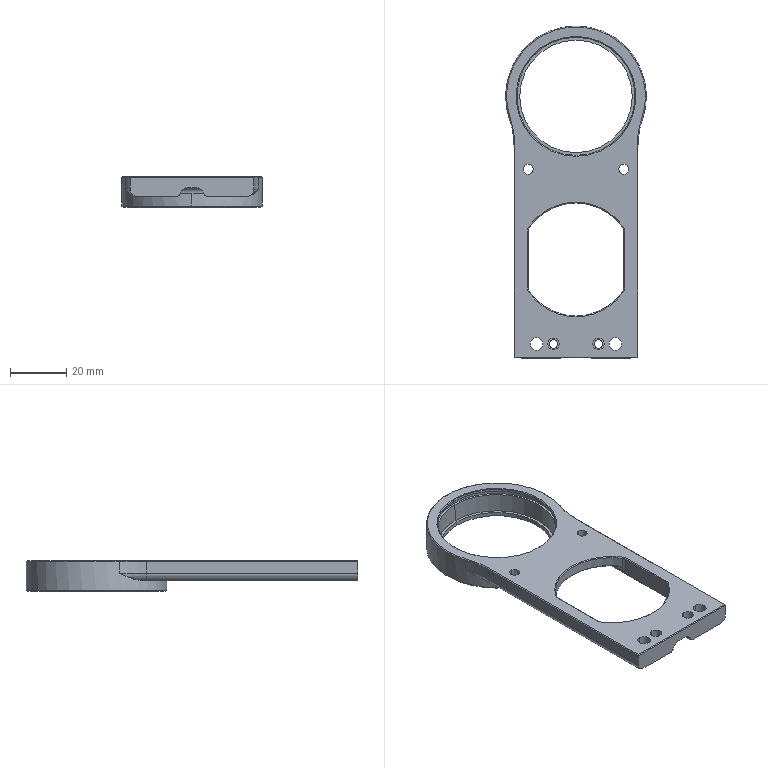NC program | NX | posted with a generic post | part box 50 x 118 x 11 mm
Lines 9691 to 9841 of 9841:
(PLANAR_MILL_2 , TOOL : D6A45)
N19326 T01 M6
N19328 G54
N19330 G17 G0 G90 X110.803 Y-1.297 S9500 M3
N19332 G43 Z30. H1
N19334 Z0.5
N19336 G94 G1 Z-1. F1250.
N19338 X111.55 Y-0.866
N19340 G3 X112.05 Y0. R1.
N19342 X93. Y19.05 R19.05
N19344 X112.05 Y0. R-19.05
N19346 X111.55 Y0.866 R1.
N19348 G1 X110.803 Y1.297
N19350 Z0.5
N19352 G0 Z30.
(PLANAR_MILL_2_COPY , TOOL : D6A45)
N19354 X66.329 Y-1.253
N19356 Z0.5
N19358 G1 Z-1.
N19360 X67. Y-0.866
N19362 G3 X67.5 Y0. R1.
N19364 G2 X93. Y25.5 R25.5
N19366 X67.5 Y0. R-25.5
N19368 G3 X67. Y0.866 R1.
N19370 G1 X66.329 Y1.253
N19372 Z0.5
N19374 G0 Z30.
(PLANAR_MILL_2_COPY_1 , TOOL : D6A45)
N19376 X4.45 Y-7.867
N19378 Z-4.
N19380 G1 Y-8.184 Z-4.085
N19382 X4.59 Y-8.41 Z-4.156
N19384 X4.816 Y-8.55 Z-4.227
N19386 X5.184 Z-4.326
N19388 X5.41 Y-8.41 Z-4.397
N19390 X5.55 Y-8.184 Z-4.468
N19392 Y-7.816 Z-4.567
N19394 X5.41 Y-7.59 Z-4.638
N19396 X5.184 Y-7.45 Z-4.71
N19398 X4.816 Z-4.808
N19400 X4.59 Y-7.59 Z-4.879
N19402 X4.45 Y-7.816 Z-4.951
N19404 Y-8. Z-5.
N19406 G3 X5. Y-8.55 R0.55
N19408 X4.45 Y-8. R-0.55
N19410 X4.517 Y-8.25 R0.5
N19412 G1 Z-4.
N19414 G0 Z30.
N19416 X3.756 Y-13.475
N19418 Z-4.
N19420 G1 Z-5.
N19422 X2.95 Y-13.134
N19424 G3 X2.45 Y-14. R1.
N19426 X5. Y-16.55 R2.55
N19428 X2.45 Y-14. R-2.55
N19430 X2.95 Y-14.866 R1.
N19432 G1 X3.756 Y-14.525
N19434 Z-4.
N19436 G0 Z30.
N19438 X-2.15 Y-20.77
N19440 Z-4.
N19442 G1 Z-5.
N19444 X-1.45 Y-20.366
N19446 G3 X-0.95 Y-19.5 R1.
N19448 G1 Y-5.373
N19450 G3 X-1.45 Y-4.507 R1.
N19452 G1 X-2.15 Y-4.103
N19454 Z-4.
N19456 G0 Z30.
N19458 Y4.103
N19460 Z-4.
N19462 G1 Z-5.
N19464 X-1.45 Y4.507
N19466 G3 X-0.95 Y5.373 R1.
N19468 G1 Y19.5
N19470 G3 X-1.45 Y20.366 R1.
N19472 G1 X-2.15 Y20.77
N19474 Z-4.
N19476 G0 Z30.
N19478 X6.244 Y13.475
N19480 Z-4.
N19482 G1 Z-5.
N19484 X7.05 Y13.134
N19486 G3 X7.55 Y14. R1.
N19488 X5. Y16.55 R2.55
N19490 X7.55 Y14. R-2.55
N19492 X7.05 Y14.866 R1.
N19494 G1 X6.244 Y14.525
N19496 Z-4.
N19498 G0 Z30.
N19500 X5.55 Y7.867
N19502 Z-4.
N19504 G1 Y8.184 Z-4.085
N19506 X5.41 Y8.41 Z-4.156
N19508 X5.184 Y8.55 Z-4.227
N19510 X4.816 Z-4.326
N19512 X4.59 Y8.41 Z-4.397
N19514 X4.45 Y8.184 Z-4.468
N19516 Y7.816 Z-4.567
N19518 X4.59 Y7.59 Z-4.638
N19520 X4.816 Y7.45 Z-4.71
N19522 X5.184 Z-4.808
N19524 X5.41 Y7.59 Z-4.879
N19526 X5.55 Y7.816 Z-4.951
N19528 Y8. Z-5.
N19530 G3 X5. Y8.55 R0.55
N19532 X5.55 Y8. R-0.55
N19534 G1 Z-4.
N19536 G0 Z30.
N19538 X66.949 Y17.8
N19540 Z-4.
N19542 G1 X66.862 Z-4.023
N19544 X66.497 Y17.587 Z-4.137
N19546 X66.284 Y17.221 Z-4.25
N19548 Y16.779 Z-4.369
N19550 X66.497 Y16.413 Z-4.482
N19552 X66.862 Y16.2 Z-4.595
N19554 X67.305 Z-4.714
N19556 X67.67 Y16.413 Z-4.827
N19558 X67.884 Y16.779 Z-4.941
N19560 Y17. Z-5.
N19562 G3 X67.084 Y17.8 R0.8
N19564 X67.884 Y17. R-0.8
N19566 X66.918 Y16.741 R1.
N19568 G1 Z-4.
N19570 G0 Z30.
N19572 X67.218 Y-17.8
N19574 Z-4.
N19576 G1 X67.305 Z-4.023
N19578 X67.67 Y-17.587 Z-4.137
N19580 X67.884 Y-17.221 Z-4.25
N19582 Y-16.779 Z-4.369
N19584 X67.67 Y-16.413 Z-4.482
N19586 X67.305 Y-16.2 Z-4.595
N19588 X66.862 Z-4.714
N19590 X66.497 Y-16.413 Z-4.827
N19592 X66.284 Y-16.779 Z-4.941
N19594 Y-17. Z-5.
N19596 G3 X67.084 Y-17.8 R0.8
N19598 X66.284 Y-17. R-0.8
N19600 X67.249 Y-16.741 R1.
N19602 G1 Z-4.
N19604 G0 Z30.
N19606 M5
N19608 M2